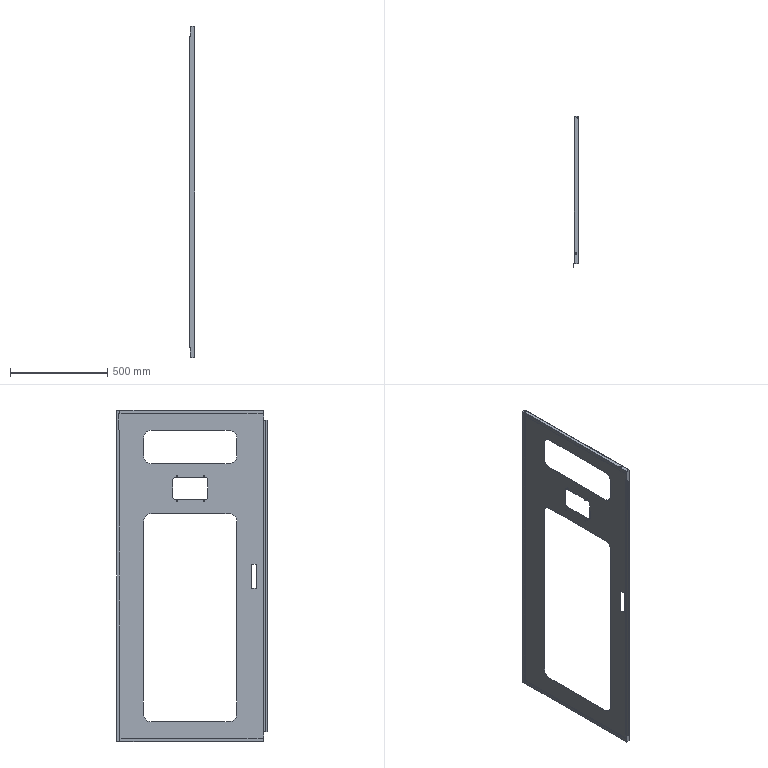Part | STEP file | RJWD-DY-0103_X2_53F367DC95E8_48 | 1 solid | 207 faces | box 26.5 x 775.2 x 1704 mm | volume 873122 mm3 | plane 124 | cylinder 75 | cone 8 | commonest cylinder face diameters 3 x30 0.4 x8 2.4 x8 4 x8 80 x8 9 x4